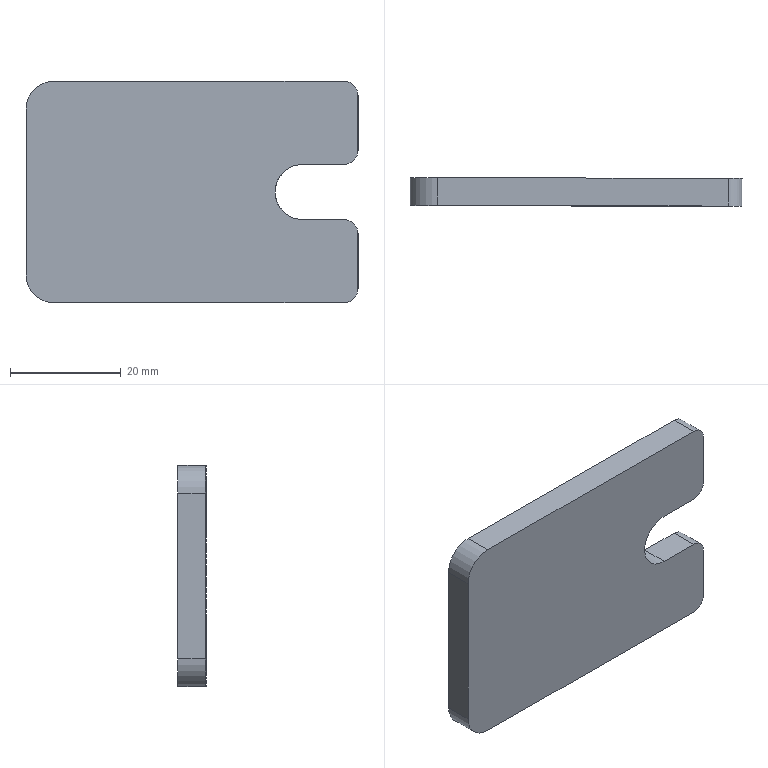Part | STEP file | Input 43 | 1 solid | 16 faces | box 60.015 x 5.178 x 40 mm | volume 11223 mm3 | plane 9 | cylinder 7 | commonest cylinder face diameters 5 x4 10 x3
STEP:
#1=CARTESIAN_POINT('',(0.,0.,0.));
#2=DIRECTION('',(0.,0.,1.));
#3=DIRECTION('',(1.,0.,0.));
#4=AXIS2_PLACEMENT_3D('',#1,#2,#3);
#5=CARTESIAN_POINT('',(-3018.306,387.735,-155.745));
#6=VERTEX_POINT('',#5);
#7=CARTESIAN_POINT('',(-3018.321,382.735,-155.745));
#8=VERTEX_POINT('',#7);
#9=CARTESIAN_POINT('',(-3018.306,387.735,-155.745));
#10=DIRECTION('',(-0.002971,-1.,0.));
#11=VECTOR('',#10,1.);
#12=LINE('',#9,#11);
#13=CARTESIAN_POINT('',(-3018.306,387.735,-160.745));
#14=DIRECTION('',(-0.002971,-1.,0.));
#15=DIRECTION('',(1.,-0.002971,0.));
#16=AXIS2_PLACEMENT_3D('',#13,#14,#15);
#17=CYLINDRICAL_SURFACE('',#16,5.);
#18=CARTESIAN_POINT('',(1.571,0.));
#19=DIRECTION('',(0.,1.));
#20=VECTOR('',#19,1.);
#21=LINE('',#18,#20);
#22=(GEOMETRIC_REPRESENTATION_CONTEXT(2)PARAMETRIC_REPRESENTATION_CONTEXT()REPRESENTATION_CONTEXT('',''));
#23=DEFINITIONAL_REPRESENTATION('',(#21),#22);
#24=PCURVE('',#17,#23);
#25=CARTESIAN_POINT('',(-3018.306,387.735,-155.745));
#26=DIRECTION('',(0.,0.,1.));
#27=DIRECTION('',(1.,-0.002971,0.));
#28=AXIS2_PLACEMENT_3D('',#25,#26,#27);
#29=PLANE('',#28);
#30=CARTESIAN_POINT('',(0.,0.));
#31=DIRECTION('',(0.,-1.));
#32=VECTOR('',#31,1.);
#33=LINE('',#30,#32);
#34=(GEOMETRIC_REPRESENTATION_CONTEXT(2)PARAMETRIC_REPRESENTATION_CONTEXT()REPRESENTATION_CONTEXT('',''));
#35=DEFINITIONAL_REPRESENTATION('',(#33),#34);
#36=PCURVE('',#29,#35);
#37=SURFACE_CURVE('',#12,(#24,#36),.PCURVE_S1.);
#38=EDGE_CURVE('',#6,#8,#37,.T.);
#39=ORIENTED_EDGE('',*,*,#38,.F.);
#40=CARTESIAN_POINT('',(-3018.306,387.735,-165.745));
#41=VERTEX_POINT('',#40);
#42=CARTESIAN_POINT('',(-3018.306,387.735,-160.745));
#43=DIRECTION('',(-0.002971,-1.,0.));
#44=DIRECTION('',(-1.,0.002971,0.));
#45=AXIS2_PLACEMENT_3D('',#42,#43,#44);
#46=CIRCLE('',#45,5.);
#47=CARTESIAN_POINT('',(-3.142,0.));
#48=DIRECTION('',(1.,0.));
#49=VECTOR('',#48,1.);
#50=LINE('',#47,#49);
#51=(GEOMETRIC_REPRESENTATION_CONTEXT(2)PARAMETRIC_REPRESENTATION_CONTEXT()REPRESENTATION_CONTEXT('',''));
#52=DEFINITIONAL_REPRESENTATION('',(#50),#51);
#53=PCURVE('',#17,#52);
#54=CARTESIAN_POINT('',(-3018.306,387.735,-160.745));
#55=DIRECTION('',(0.002971,1.,0.));
#56=DIRECTION('',(-1.,0.002971,0.));
#57=AXIS2_PLACEMENT_3D('',#54,#55,#56);
#58=PLANE('',#57);
#59=CARTESIAN_POINT('',(5.,0.));
#60=CARTESIAN_POINT('',(5.,-8.66));
#61=CARTESIAN_POINT('',(-2.5,-4.33));
#62=CARTESIAN_POINT('',(-10.,0.));
#63=CARTESIAN_POINT('',(-2.5,4.33));
#64=CARTESIAN_POINT('',(5.,8.66));
#65=CARTESIAN_POINT('',(5.,0.));
#66=(BOUNDED_CURVE()B_SPLINE_CURVE(2,(#59,#60,#61,#62,#63,#64,#65),.UNSPECIFIED.,.T.,.F.)B_SPLINE_CURVE_WITH_KNOTS((1,2,2,2,2,1),(-2.094,0.,2.094,4.189,6.283,8.378),.UNSPECIFIED.)CURVE()GEOMETRIC_REPRESENTATION_ITEM()RATIONAL_B_SPLINE_CURVE((1.,0.5,1.,0.5,1.,0.5,1.))REPRESENTATION_ITEM(''));
#67=(GEOMETRIC_REPRESENTATION_CONTEXT(2)PARAMETRIC_REPRESENTATION_CONTEXT()REPRESENTATION_CONTEXT('',''));
#68=DEFINITIONAL_REPRESENTATION('',(#66),#67);
#69=PCURVE('',#58,#68);
#70=SURFACE_CURVE('',#46,(#53,#69),.PCURVE_S1.);
#71=EDGE_CURVE('',#6,#41,#70,.T.);
#72=ORIENTED_EDGE('',*,*,#71,.T.);
#73=CARTESIAN_POINT('',(-3018.321,382.735,-165.745));
#74=VERTEX_POINT('',#73);
#75=CARTESIAN_POINT('',(-3018.306,387.735,-165.745));
#76=DIRECTION('',(-0.002971,-1.,0.));
#77=VECTOR('',#76,1.);
#78=LINE('',#75,#77);
#79=CARTESIAN_POINT('',(4.712,0.));
#80=DIRECTION('',(0.,1.));
#81=VECTOR('',#80,1.);
#82=LINE('',#79,#81);
#83=(GEOMETRIC_REPRESENTATION_CONTEXT(2)PARAMETRIC_REPRESENTATION_CONTEXT()REPRESENTATION_CONTEXT('',''));
#84=DEFINITIONAL_REPRESENTATION('',(#82),#83);
#85=PCURVE('',#17,#84);
#86=CARTESIAN_POINT('',(-3018.306,387.735,-165.745));
#87=DIRECTION('',(0.,0.,-1.));
#88=DIRECTION('',(-1.,0.002971,0.));
#89=AXIS2_PLACEMENT_3D('',#86,#87,#88);
#90=PLANE('',#89);
#91=CARTESIAN_POINT('',(0.,0.));
#92=DIRECTION('',(0.,-1.));
#93=VECTOR('',#92,1.);
#94=LINE('',#91,#93);
#95=(GEOMETRIC_REPRESENTATION_CONTEXT(2)PARAMETRIC_REPRESENTATION_CONTEXT()REPRESENTATION_CONTEXT('',''));
#96=DEFINITIONAL_REPRESENTATION('',(#94),#95);
#97=PCURVE('',#90,#96);
#98=SURFACE_CURVE('',#78,(#85,#97),.PCURVE_S1.);
#99=EDGE_CURVE('',#41,#74,#98,.T.);
#100=ORIENTED_EDGE('',*,*,#99,.T.);
#101=CARTESIAN_POINT('',(-3018.321,382.735,-160.745));
#102=DIRECTION('',(-0.002971,-1.,0.));
#103=DIRECTION('',(-1.,0.002971,0.));
#104=AXIS2_PLACEMENT_3D('',#101,#102,#103);
#105=CIRCLE('',#104,5.);
#106=CARTESIAN_POINT('',(-3.142,5.));
#107=DIRECTION('',(1.,0.));
#108=VECTOR('',#107,1.);
#109=LINE('',#106,#108);
#110=(GEOMETRIC_REPRESENTATION_CONTEXT(2)PARAMETRIC_REPRESENTATION_CONTEXT()REPRESENTATION_CONTEXT('',''));
#111=DEFINITIONAL_REPRESENTATION('',(#109),#110);
#112=PCURVE('',#17,#111);
#113=CARTESIAN_POINT('',(-3018.321,382.735,-160.745));
#114=DIRECTION('',(0.002971,1.,0.));
#115=DIRECTION('',(-1.,0.002971,0.));
#116=AXIS2_PLACEMENT_3D('',#113,#114,#115);
#117=PLANE('',#116);
#118=CARTESIAN_POINT('',(5.,0.));
#119=CARTESIAN_POINT('',(5.,-8.66));
#120=CARTESIAN_POINT('',(-2.5,-4.33));
#121=CARTESIAN_POINT('',(-10.,0.));
#122=CARTESIAN_POINT('',(-2.5,4.33));
#123=CARTESIAN_POINT('',(5.,8.66));
#124=CARTESIAN_POINT('',(5.,0.));
#125=(BOUNDED_CURVE()B_SPLINE_CURVE(2,(#118,#119,#120,#121,#122,#123,#124),.UNSPECIFIED.,.T.,.F.)B_SPLINE_CURVE_WITH_KNOTS((1,2,2,2,2,1),(-2.094,0.,2.094,4.189,6.283,8.378),.UNSPECIFIED.)CURVE()GEOMETRIC_REPRESENTATION_ITEM()RATIONAL_B_SPLINE_CURVE((1.,0.5,1.,0.5,1.,0.5,1.))REPRESENTATION_ITEM(''));
#126=(GEOMETRIC_REPRESENTATION_CONTEXT(2)PARAMETRIC_REPRESENTATION_CONTEXT()REPRESENTATION_CONTEXT('',''));
#127=DEFINITIONAL_REPRESENTATION('',(#125),#126);
#128=PCURVE('',#117,#127);
#129=SURFACE_CURVE('',#105,(#112,#128),.PCURVE_S1.);
#130=EDGE_CURVE('',#8,#74,#129,.T.);
#131=ORIENTED_EDGE('',*,*,#130,.F.);
#132=EDGE_LOOP('',(#39,#72,#100,#131));
#133=FACE_BOUND('',#132,.F.);
#134=ADVANCED_FACE('',(#133),#17,.F.);
#135=CARTESIAN_POINT('',(-3010.821,382.713,-165.745));
#136=VERTEX_POINT('',#135);
#137=CARTESIAN_POINT('',(-3018.321,382.735,-165.745));
#138=DIRECTION('',(1.,-0.002971,0.));
#139=VECTOR('',#138,1.);
#140=LINE('',#137,#139);
#141=CARTESIAN_POINT('',(0.,-5.));
#142=DIRECTION('',(-1.,0.));
#143=VECTOR('',#142,1.);
#144=LINE('',#141,#143);
#145=(GEOMETRIC_REPRESENTATION_CONTEXT(2)PARAMETRIC_REPRESENTATION_CONTEXT()REPRESENTATION_CONTEXT('',''));
#146=DEFINITIONAL_REPRESENTATION('',(#144),#145);
#147=PCURVE('',#90,#146);
#148=CARTESIAN_POINT('',(0.,-5.));
#149=DIRECTION('',(-1.,0.));
#150=VECTOR('',#149,1.);
#151=LINE('',#148,#150);
#152=(GEOMETRIC_REPRESENTATION_CONTEXT(2)PARAMETRIC_REPRESENTATION_CONTEXT()REPRESENTATION_CONTEXT('',''));
#153=DEFINITIONAL_REPRESENTATION('',(#151),#152);
#154=PCURVE('',#117,#153);
#155=SURFACE_CURVE('',#140,(#147,#154),.PCURVE_S1.);
#156=EDGE_CURVE('',#74,#136,#155,.T.);
#157=ORIENTED_EDGE('',*,*,#156,.T.);
#158=CARTESIAN_POINT('',(-3010.806,387.713,-165.745));
#159=VERTEX_POINT('',#158);
#160=CARTESIAN_POINT('',(-3010.806,387.713,-165.745));
#161=DIRECTION('',(-0.002971,-1.,0.));
#162=VECTOR('',#161,1.);
#163=LINE('',#160,#162);
#164=CARTESIAN_POINT('',(-7.5,0.));
#165=DIRECTION('',(0.,-1.));
#166=VECTOR('',#165,1.);
#167=LINE('',#164,#166);
#168=(GEOMETRIC_REPRESENTATION_CONTEXT(2)PARAMETRIC_REPRESENTATION_CONTEXT()REPRESENTATION_CONTEXT('',''));
#169=DEFINITIONAL_REPRESENTATION('',(#167),#168);
#170=PCURVE('',#90,#169);
#171=CARTESIAN_POINT('',(-3010.806,387.713,-168.245));
#172=DIRECTION('',(-0.002971,-1.,0.));
#173=DIRECTION('',(1.,-0.002971,0.));
#174=AXIS2_PLACEMENT_3D('',#171,#172,#173);
#175=CYLINDRICAL_SURFACE('',#174,2.5);
#176=CARTESIAN_POINT('',(1.571,0.));
#177=DIRECTION('',(0.,1.));
#178=VECTOR('',#177,1.);
#179=LINE('',#176,#178);
#180=(GEOMETRIC_REPRESENTATION_CONTEXT(2)PARAMETRIC_REPRESENTATION_CONTEXT()REPRESENTATION_CONTEXT('',''));
#181=DEFINITIONAL_REPRESENTATION('',(#179),#180);
#182=PCURVE('',#175,#181);
#183=SURFACE_CURVE('',#163,(#170,#182),.PCURVE_S1.);
#184=EDGE_CURVE('',#159,#136,#183,.T.);
#185=ORIENTED_EDGE('',*,*,#184,.F.);
#186=CARTESIAN_POINT('',(-3018.306,387.735,-165.745));
#187=DIRECTION('',(1.,-0.002971,0.));
#188=VECTOR('',#187,1.);
#189=LINE('',#186,#188);
#190=CARTESIAN_POINT('',(0.,0.));
#191=DIRECTION('',(-1.,0.));
#192=VECTOR('',#191,1.);
#193=LINE('',#190,#192);
#194=(GEOMETRIC_REPRESENTATION_CONTEXT(2)PARAMETRIC_REPRESENTATION_CONTEXT()REPRESENTATION_CONTEXT('',''));
#195=DEFINITIONAL_REPRESENTATION('',(#193),#194);
#196=PCURVE('',#90,#195);
#197=CARTESIAN_POINT('',(0.,-5.));
#198=DIRECTION('',(-1.,0.));
#199=VECTOR('',#198,1.);
#200=LINE('',#197,#199);
#201=(GEOMETRIC_REPRESENTATION_CONTEXT(2)PARAMETRIC_REPRESENTATION_CONTEXT()REPRESENTATION_CONTEXT('',''));
#202=DEFINITIONAL_REPRESENTATION('',(#200),#201);
#203=PCURVE('',#58,#202);
#204=SURFACE_CURVE('',#189,(#196,#203),.PCURVE_S1.);
#205=EDGE_CURVE('',#41,#159,#204,.T.);
#206=ORIENTED_EDGE('',*,*,#205,.F.);
#207=ORIENTED_EDGE('',*,*,#99,.T.);
#208=EDGE_LOOP('',(#157,#185,#206,#207));
#209=FACE_BOUND('',#208,.T.);
#210=ADVANCED_FACE('',(#209),#90,.F.);
#211=CARTESIAN_POINT('',(-3008.321,382.706,-168.245));
#212=VERTEX_POINT('',#211);
#213=CARTESIAN_POINT('',(-3010.821,382.713,-168.245));
#214=DIRECTION('',(0.002971,1.,0.));
#215=DIRECTION('',(-1.,0.002971,0.));
#216=AXIS2_PLACEMENT_3D('',#213,#214,#215);
#217=CIRCLE('',#216,2.5);
#218=CARTESIAN_POINT('',(3.142,5.));
#219=DIRECTION('',(-1.,0.));
#220=VECTOR('',#219,1.);
#221=LINE('',#218,#220);
#222=(GEOMETRIC_REPRESENTATION_CONTEXT(2)PARAMETRIC_REPRESENTATION_CONTEXT()REPRESENTATION_CONTEXT('',''));
#223=DEFINITIONAL_REPRESENTATION('',(#221),#222);
#224=PCURVE('',#175,#223);
#225=CARTESIAN_POINT('',(-7.5,-7.5));
#226=DIRECTION('',(1.,0.));
#227=AXIS2_PLACEMENT_2D('',#225,#226);
#228=CIRCLE('',#227,2.5);
#229=(GEOMETRIC_REPRESENTATION_CONTEXT(2)PARAMETRIC_REPRESENTATION_CONTEXT()REPRESENTATION_CONTEXT('',''));
#230=DEFINITIONAL_REPRESENTATION('',(#228),#229);
#231=PCURVE('',#117,#230);
#232=SURFACE_CURVE('',#217,(#224,#231),.PCURVE_S1.);
#233=EDGE_CURVE('',#136,#212,#232,.T.);
#234=ORIENTED_EDGE('',*,*,#233,.T.);
#235=CARTESIAN_POINT('',(-3008.306,387.705,-168.245));
#236=VERTEX_POINT('',#235);
#237=CARTESIAN_POINT('',(-3008.306,387.705,-168.245));
#238=DIRECTION('',(-0.002971,-1.,0.));
#239=VECTOR('',#238,1.);
#240=LINE('',#237,#239);
#241=CARTESIAN_POINT('',(0.,0.));
#242=DIRECTION('',(0.,1.));
#243=VECTOR('',#242,1.);
#244=LINE('',#241,#243);
#245=(GEOMETRIC_REPRESENTATION_CONTEXT(2)PARAMETRIC_REPRESENTATION_CONTEXT()REPRESENTATION_CONTEXT('',''));
#246=DEFINITIONAL_REPRESENTATION('',(#244),#245);
#247=PCURVE('',#175,#246);
#248=CARTESIAN_POINT('',(-3008.306,387.705,-168.245));
#249=DIRECTION('',(-1.,0.002971,0.));
#250=DIRECTION('',(0.,0.,1.));
#251=AXIS2_PLACEMENT_3D('',#248,#249,#250);
#252=PLANE('',#251);
#253=CARTESIAN_POINT('',(0.,0.));
#254=DIRECTION('',(0.,-1.));
#255=VECTOR('',#254,1.);
#256=LINE('',#253,#255);
#257=(GEOMETRIC_REPRESENTATION_CONTEXT(2)PARAMETRIC_REPRESENTATION_CONTEXT()REPRESENTATION_CONTEXT('',''));
#258=DEFINITIONAL_REPRESENTATION('',(#256),#257);
#259=PCURVE('',#252,#258);
#260=SURFACE_CURVE('',#240,(#247,#259),.PCURVE_S1.);
#261=EDGE_CURVE('',#236,#212,#260,.T.);
#262=ORIENTED_EDGE('',*,*,#261,.F.);
#263=CARTESIAN_POINT('',(-3010.806,387.713,-168.245));
#264=DIRECTION('',(0.002971,1.,0.));
#265=DIRECTION('',(-1.,0.002971,0.));
#266=AXIS2_PLACEMENT_3D('',#263,#264,#265);
#267=CIRCLE('',#266,2.5);
#268=CARTESIAN_POINT('',(3.142,0.));
#269=DIRECTION('',(-1.,0.));
#270=VECTOR('',#269,1.);
#271=LINE('',#268,#270);
#272=(GEOMETRIC_REPRESENTATION_CONTEXT(2)PARAMETRIC_REPRESENTATION_CONTEXT()REPRESENTATION_CONTEXT('',''));
#273=DEFINITIONAL_REPRESENTATION('',(#271),#272);
#274=PCURVE('',#175,#273);
#275=CARTESIAN_POINT('',(-7.5,-7.5));
#276=DIRECTION('',(1.,0.));
#277=AXIS2_PLACEMENT_2D('',#275,#276);
#278=CIRCLE('',#277,2.5);
#279=(GEOMETRIC_REPRESENTATION_CONTEXT(2)PARAMETRIC_REPRESENTATION_CONTEXT()REPRESENTATION_CONTEXT('',''));
#280=DEFINITIONAL_REPRESENTATION('',(#278),#279);
#281=PCURVE('',#58,#280);
#282=SURFACE_CURVE('',#267,(#274,#281),.PCURVE_S1.);
#283=EDGE_CURVE('',#159,#236,#282,.T.);
#284=ORIENTED_EDGE('',*,*,#283,.F.);
#285=ORIENTED_EDGE('',*,*,#184,.T.);
#286=EDGE_LOOP('',(#234,#262,#284,#285));
#287=FACE_BOUND('',#286,.T.);
#288=ADVANCED_FACE('',(#287),#175,.T.);
#289=CARTESIAN_POINT('',(-3008.321,382.706,-178.245));
#290=VERTEX_POINT('',#289);
#291=CARTESIAN_POINT('',(-3008.321,382.706,-168.245));
#292=DIRECTION('',(0.,0.,-1.));
#293=VECTOR('',#292,1.);
#294=LINE('',#291,#293);
#295=CARTESIAN_POINT('',(0.,-5.));
#296=DIRECTION('',(-1.,0.));
#297=VECTOR('',#296,1.);
#298=LINE('',#295,#297);
#299=(GEOMETRIC_REPRESENTATION_CONTEXT(2)PARAMETRIC_REPRESENTATION_CONTEXT()REPRESENTATION_CONTEXT('',''));
#300=DEFINITIONAL_REPRESENTATION('',(#298),#299);
#301=PCURVE('',#252,#300);
#302=CARTESIAN_POINT('',(-10.,-7.5));
#303=DIRECTION('',(0.,-1.));
#304=VECTOR('',#303,1.);
#305=LINE('',#302,#304);
#306=(GEOMETRIC_REPRESENTATION_CONTEXT(2)PARAMETRIC_REPRESENTATION_CONTEXT()REPRESENTATION_CONTEXT('',''));
#307=DEFINITIONAL_REPRESENTATION('',(#305),#306);
#308=PCURVE('',#117,#307);
#309=SURFACE_CURVE('',#294,(#301,#308),.PCURVE_S1.);
#310=EDGE_CURVE('',#212,#290,#309,.T.);
#311=ORIENTED_EDGE('',*,*,#310,.T.);
#312=CARTESIAN_POINT('',(-3008.306,387.705,-178.245));
#313=VERTEX_POINT('',#312);
#314=CARTESIAN_POINT('',(-3008.306,387.705,-178.245));
#315=DIRECTION('',(-0.002971,-1.,0.));
#316=VECTOR('',#315,1.);
#317=LINE('',#314,#316);
#318=CARTESIAN_POINT('',(-10.,0.));
#319=DIRECTION('',(0.,-1.));
#320=VECTOR('',#319,1.);
#321=LINE('',#318,#320);
#322=(GEOMETRIC_REPRESENTATION_CONTEXT(2)PARAMETRIC_REPRESENTATION_CONTEXT()REPRESENTATION_CONTEXT('',''));
#323=DEFINITIONAL_REPRESENTATION('',(#321),#322);
#324=PCURVE('',#252,#323);
#325=CARTESIAN_POINT('',(-3010.806,387.713,-178.245));
#326=DIRECTION('',(-0.002971,-1.,0.));
#327=DIRECTION('',(1.,-0.002971,0.));
#328=AXIS2_PLACEMENT_3D('',#325,#326,#327);
#329=CYLINDRICAL_SURFACE('',#328,2.5);
#330=CARTESIAN_POINT('',(6.283,0.));
#331=DIRECTION('',(0.,1.));
#332=VECTOR('',#331,1.);
#333=LINE('',#330,#332);
#334=(GEOMETRIC_REPRESENTATION_CONTEXT(2)PARAMETRIC_REPRESENTATION_CONTEXT()REPRESENTATION_CONTEXT('',''));
#335=DEFINITIONAL_REPRESENTATION('',(#333),#334);
#336=PCURVE('',#329,#335);
#337=SURFACE_CURVE('',#317,(#324,#336),.PCURVE_S1.);
#338=EDGE_CURVE('',#313,#290,#337,.T.);
#339=ORIENTED_EDGE('',*,*,#338,.F.);
#340=CARTESIAN_POINT('',(-3008.306,387.705,-168.245));
#341=DIRECTION('',(0.,0.,-1.));
#342=VECTOR('',#341,1.);
#343=LINE('',#340,#342);
#344=CARTESIAN_POINT('',(0.,0.));
#345=DIRECTION('',(-1.,0.));
#346=VECTOR('',#345,1.);
#347=LINE('',#344,#346);
#348=(GEOMETRIC_REPRESENTATION_CONTEXT(2)PARAMETRIC_REPRESENTATION_CONTEXT()REPRESENTATION_CONTEXT('',''));
#349=DEFINITIONAL_REPRESENTATION('',(#347),#348);
#350=PCURVE('',#252,#349);
#351=CARTESIAN_POINT('',(-10.,-7.5));
#352=DIRECTION('',(0.,-1.));
#353=VECTOR('',#352,1.);
#354=LINE('',#351,#353);
#355=(GEOMETRIC_REPRESENTATION_CONTEXT(2)PARAMETRIC_REPRESENTATION_CONTEXT()REPRESENTATION_CONTEXT('',''));
#356=DEFINITIONAL_REPRESENTATION('',(#354),#355);
#357=PCURVE('',#58,#356);
#358=SURFACE_CURVE('',#343,(#350,#357),.PCURVE_S1.);
#359=EDGE_CURVE('',#236,#313,#358,.T.);
#360=ORIENTED_EDGE('',*,*,#359,.F.);
#361=ORIENTED_EDGE('',*,*,#261,.T.);
#362=EDGE_LOOP('',(#311,#339,#360,#361));
#363=FACE_BOUND('',#362,.T.);
#364=ADVANCED_FACE('',(#363),#252,.F.);
#365=CARTESIAN_POINT('',(-3010.821,382.713,-180.745));
#366=VERTEX_POINT('',#365);
#367=CARTESIAN_POINT('',(-3010.821,382.713,-178.245));
#368=DIRECTION('',(0.002971,1.,0.));
#369=DIRECTION('',(-1.,0.002971,0.));
#370=AXIS2_PLACEMENT_3D('',#367,#368,#369);
#371=CIRCLE('',#370,2.5);
#372=CARTESIAN_POINT('',(9.425,5.));
#373=DIRECTION('',(-1.,0.));
#374=VECTOR('',#373,1.);
#375=LINE('',#372,#374);
#376=(GEOMETRIC_REPRESENTATION_CONTEXT(2)PARAMETRIC_REPRESENTATION_CONTEXT()REPRESENTATION_CONTEXT('',''));
#377=DEFINITIONAL_REPRESENTATION('',(#375),#376);
#378=PCURVE('',#329,#377);
#379=CARTESIAN_POINT('',(-7.5,-17.5));
#380=DIRECTION('',(1.,0.));
#381=AXIS2_PLACEMENT_2D('',#379,#380);
#382=CIRCLE('',#381,2.5);
#383=(GEOMETRIC_REPRESENTATION_CONTEXT(2)PARAMETRIC_REPRESENTATION_CONTEXT()REPRESENTATION_CONTEXT('',''));
#384=DEFINITIONAL_REPRESENTATION('',(#382),#383);
#385=PCURVE('',#117,#384);
#386=SURFACE_CURVE('',#371,(#378,#385),.PCURVE_S1.);
#387=EDGE_CURVE('',#290,#366,#386,.T.);
#388=ORIENTED_EDGE('',*,*,#387,.T.);
#389=CARTESIAN_POINT('',(-3010.806,387.713,-180.745));
#390=VERTEX_POINT('',#389);
#391=CARTESIAN_POINT('',(-3010.806,387.713,-180.745));
#392=DIRECTION('',(-0.002971,-1.,0.));
#393=VECTOR('',#392,1.);
#394=LINE('',#391,#393);
#395=CARTESIAN_POINT('',(4.712,0.));
#396=DIRECTION('',(0.,1.));
#397=VECTOR('',#396,1.);
#398=LINE('',#395,#397);
#399=(GEOMETRIC_REPRESENTATION_CONTEXT(2)PARAMETRIC_REPRESENTATION_CONTEXT()REPRESENTATION_CONTEXT('',''));
#400=DEFINITIONAL_REPRESENTATION('',(#398),#399);
#401=PCURVE('',#329,#400);
#402=CARTESIAN_POINT('',(-3010.806,387.713,-180.745));
#403=DIRECTION('',(0.,0.,1.));
#404=DIRECTION('',(1.,-0.002971,0.));
#405=AXIS2_PLACEMENT_3D('',#402,#403,#404);
#406=PLANE('',#405);
#407=CARTESIAN_POINT('',(0.,0.));
#408=DIRECTION('',(0.,-1.));
#409=VECTOR('',#408,1.);
#410=LINE('',#407,#409);
#411=(GEOMETRIC_REPRESENTATION_CONTEXT(2)PARAMETRIC_REPRESENTATION_CONTEXT()REPRESENTATION_CONTEXT('',''));
#412=DEFINITIONAL_REPRESENTATION('',(#410),#411);
#413=PCURVE('',#406,#412);
#414=SURFACE_CURVE('',#394,(#401,#413),.PCURVE_S1.);
#415=EDGE_CURVE('',#390,#366,#414,.T.);
#416=ORIENTED_EDGE('',*,*,#415,.F.);
#417=CARTESIAN_POINT('',(-3010.806,387.713,-178.245));
#418=DIRECTION('',(0.002971,1.,0.));
#419=DIRECTION('',(-1.,0.002971,0.));
#420=AXIS2_PLACEMENT_3D('',#417,#418,#419);
#421=CIRCLE('',#420,2.5);
#422=CARTESIAN_POINT('',(9.425,0.));
#423=DIRECTION('',(-1.,0.));
#424=VECTOR('',#423,1.);
#425=LINE('',#422,#424);
#426=(GEOMETRIC_REPRESENTATION_CONTEXT(2)PARAMETRIC_REPRESENTATION_CONTEXT()REPRESENTATION_CONTEXT('',''));
#427=DEFINITIONAL_REPRESENTATION('',(#425),#426);
#428=PCURVE('',#329,#427);
#429=CARTESIAN_POINT('',(-7.5,-17.5));
#430=DIRECTION('',(1.,0.));
#431=AXIS2_PLACEMENT_2D('',#429,#430);
#432=CIRCLE('',#431,2.5);
#433=(GEOMETRIC_REPRESENTATION_CONTEXT(2)PARAMETRIC_REPRESENTATION_CONTEXT()REPRESENTATION_CONTEXT('',''));
#434=DEFINITIONAL_REPRESENTATION('',(#432),#433);
#435=PCURVE('',#58,#434);
#436=SURFACE_CURVE('',#421,(#428,#435),.PCURVE_S1.);
#437=EDGE_CURVE('',#313,#390,#436,.T.);
#438=ORIENTED_EDGE('',*,*,#437,.F.);
#439=ORIENTED_EDGE('',*,*,#338,.T.);
#440=EDGE_LOOP('',(#388,#416,#438,#439));
#441=FACE_BOUND('',#440,.T.);
#442=ADVANCED_FACE('',(#441),#329,.T.);
#443=CARTESIAN_POINT('',(-3063.321,382.869,-180.745));
#444=VERTEX_POINT('',#443);
#445=CARTESIAN_POINT('',(-3010.821,382.713,-180.745));
#446=DIRECTION('',(-1.,0.002971,0.));
#447=VECTOR('',#446,1.);
#448=LINE('',#445,#447);
#449=CARTESIAN_POINT('',(0.,-5.));
#450=DIRECTION('',(-1.,0.));
#451=VECTOR('',#450,1.);
#452=LINE('',#449,#451);
#453=(GEOMETRIC_REPRESENTATION_CONTEXT(2)PARAMETRIC_REPRESENTATION_CONTEXT()REPRESENTATION_CONTEXT('',''));
#454=DEFINITIONAL_REPRESENTATION('',(#452),#453);
#455=PCURVE('',#406,#454);
#456=CARTESIAN_POINT('',(-7.5,-20.));
#457=DIRECTION('',(1.,0.));
#458=VECTOR('',#457,1.);
#459=LINE('',#456,#458);
#460=(GEOMETRIC_REPRESENTATION_CONTEXT(2)PARAMETRIC_REPRESENTATION_CONTEXT()REPRESENTATION_CONTEXT('',''));
#461=DEFINITIONAL_REPRESENTATION('',(#459),#460);
#462=PCURVE('',#117,#461);
#463=SURFACE_CURVE('',#448,(#455,#462),.PCURVE_S1.);
#464=EDGE_CURVE('',#366,#444,#463,.T.);
#465=ORIENTED_EDGE('',*,*,#464,.T.);
#466=CARTESIAN_POINT('',(-3063.306,387.869,-180.745));
#467=VERTEX_POINT('',#466);
#468=CARTESIAN_POINT('',(-3063.306,387.869,-180.745));
#469=DIRECTION('',(-0.002971,-1.,0.));
#470=VECTOR('',#469,1.);
#471=LINE('',#468,#470);
#472=CARTESIAN_POINT('',(-52.5,0.));
#473=DIRECTION('',(0.,-1.));
#474=VECTOR('',#473,1.);
#475=LINE('',#472,#474);
#476=(GEOMETRIC_REPRESENTATION_CONTEXT(2)PARAMETRIC_REPRESENTATION_CONTEXT()REPRESENTATION_CONTEXT('',''));
#477=DEFINITIONAL_REPRESENTATION('',(#475),#476);
#478=PCURVE('',#406,#477);
#479=CARTESIAN_POINT('',(-3063.306,387.869,-175.745));
#480=DIRECTION('',(-0.002971,-1.,0.));
#481=DIRECTION('',(1.,-0.002971,0.));
#482=AXIS2_PLACEMENT_3D('',#479,#480,#481);
#483=CYLINDRICAL_SURFACE('',#482,5.);
#484=CARTESIAN_POINT('',(4.712,0.));
#485=DIRECTION('',(0.,1.));
#486=VECTOR('',#485,1.);
#487=LINE('',#484,#486);
#488=(GEOMETRIC_REPRESENTATION_CONTEXT(2)PARAMETRIC_REPRESENTATION_CONTEXT()REPRESENTATION_CONTEXT('',''));
#489=DEFINITIONAL_REPRESENTATION('',(#487),#488);
#490=PCURVE('',#483,#489);
#491=SURFACE_CURVE('',#471,(#478,#490),.PCURVE_S1.);
#492=EDGE_CURVE('',#467,#444,#491,.T.);
#493=ORIENTED_EDGE('',*,*,#492,.F.);
#494=CARTESIAN_POINT('',(-3010.806,387.713,-180.745));
#495=DIRECTION('',(-1.,0.002971,0.));
#496=VECTOR('',#495,1.);
#497=LINE('',#494,#496);
#498=CARTESIAN_POINT('',(0.,0.));
#499=DIRECTION('',(-1.,0.));
#500=VECTOR('',#499,1.);
#501=LINE('',#498,#500);
#502=(GEOMETRIC_REPRESENTATION_CONTEXT(2)PARAMETRIC_REPRESENTATION_CONTEXT()REPRESENTATION_CONTEXT('',''));
#503=DEFINITIONAL_REPRESENTATION('',(#501),#502);
#504=PCURVE('',#406,#503);
#505=CARTESIAN_POINT('',(-7.5,-20.));
#506=DIRECTION('',(1.,0.));
#507=VECTOR('',#506,1.);
#508=LINE('',#505,#507);
#509=(GEOMETRIC_REPRESENTATION_CONTEXT(2)PARAMETRIC_REPRESENTATION_CONTEXT()REPRESENTATION_CONTEXT('',''));
#510=DEFINITIONAL_REPRESENTATION('',(#508),#509);
#511=PCURVE('',#58,#510);
#512=SURFACE_CURVE('',#497,(#504,#511),.PCURVE_S1.);
#513=EDGE_CURVE('',#390,#467,#512,.T.);
#514=ORIENTED_EDGE('',*,*,#513,.F.);
#515=ORIENTED_EDGE('',*,*,#415,.T.);
#516=EDGE_LOOP('',(#465,#493,#514,#515));
#517=FACE_BOUND('',#516,.T.);
#518=ADVANCED_FACE('',(#517),#406,.F.);
#519=CARTESIAN_POINT('',(-3068.321,382.884,-175.745));
#520=VERTEX_POINT('',#519);
#521=CARTESIAN_POINT('',(-3063.321,382.869,-175.745));
#522=DIRECTION('',(0.002971,1.,0.));
#523=DIRECTION('',(1.,-0.002971,0.));
#524=AXIS2_PLACEMENT_3D('',#521,#522,#523);
#525=CIRCLE('',#524,5.);
#526=CARTESIAN_POINT('',(6.283,5.));
#527=DIRECTION('',(-1.,0.));
#528=VECTOR('',#527,1.);
#529=LINE('',#526,#528);
#530=(GEOMETRIC_REPRESENTATION_CONTEXT(2)PARAMETRIC_REPRESENTATION_CONTEXT()REPRESENTATION_CONTEXT('',''));
#531=DEFINITIONAL_REPRESENTATION('',(#529),#530);
#532=PCURVE('',#483,#531);
#533=CARTESIAN_POINT('',(45.,-15.));
#534=DIRECTION('',(-1.,0.));
#535=AXIS2_PLACEMENT_2D('',#533,#534);
#536=CIRCLE('',#535,5.);
#537=(GEOMETRIC_REPRESENTATION_CONTEXT(2)PARAMETRIC_REPRESENTATION_CONTEXT()REPRESENTATION_CONTEXT('',''));
#538=DEFINITIONAL_REPRESENTATION('',(#536),#537);
#539=PCURVE('',#117,#538);
#540=SURFACE_CURVE('',#525,(#532,#539),.PCURVE_S1.);
#541=EDGE_CURVE('',#444,#520,#540,.T.);
#542=ORIENTED_EDGE('',*,*,#541,.T.);
#543=CARTESIAN_POINT('',(-3068.306,387.884,-175.745));
#544=VERTEX_POINT('',#543);
#545=CARTESIAN_POINT('',(-3068.306,387.884,-175.745));
#546=DIRECTION('',(-0.002971,-1.,0.));
#547=VECTOR('',#546,1.);
#548=LINE('',#545,#547);
#549=CARTESIAN_POINT('',(3.142,0.));
#550=DIRECTION('',(0.,1.));
#551=VECTOR('',#550,1.);
#552=LINE('',#549,#551);
#553=(GEOMETRIC_REPRESENTATION_CONTEXT(2)PARAMETRIC_REPRESENTATION_CONTEXT()REPRESENTATION_CONTEXT('',''));
#554=DEFINITIONAL_REPRESENTATION('',(#552),#553);
#555=PCURVE('',#483,#554);
#556=CARTESIAN_POINT('',(-3068.306,387.884,-175.745));
#557=DIRECTION('',(1.,-0.002971,0.));
#558=DIRECTION('',(0.,0.,-1.));
#559=AXIS2_PLACEMENT_3D('',#556,#557,#558);
#560=PLANE('',#559);
#561=CARTESIAN_POINT('',(0.,0.));
#562=DIRECTION('',(0.,-1.));
#563=VECTOR('',#562,1.);
#564=LINE('',#561,#563);
#565=(GEOMETRIC_REPRESENTATION_CONTEXT(2)PARAMETRIC_REPRESENTATION_CONTEXT()REPRESENTATION_CONTEXT('',''));
#566=DEFINITIONAL_REPRESENTATION('',(#564),#565);
#567=PCURVE('',#560,#566);
#568=SURFACE_CURVE('',#548,(#555,#567),.PCURVE_S1.);
#569=EDGE_CURVE('',#544,#520,#568,.T.);
#570=ORIENTED_EDGE('',*,*,#569,.F.);
#571=CARTESIAN_POINT('',(-3063.306,387.869,-175.745));
#572=DIRECTION('',(0.002971,1.,0.));
#573=DIRECTION('',(1.,-0.002971,0.));
#574=AXIS2_PLACEMENT_3D('',#571,#572,#573);
#575=CIRCLE('',#574,5.);
#576=CARTESIAN_POINT('',(6.283,0.));
#577=DIRECTION('',(-1.,0.));
#578=VECTOR('',#577,1.);
#579=LINE('',#576,#578);
#580=(GEOMETRIC_REPRESENTATION_CONTEXT(2)PARAMETRIC_REPRESENTATION_CONTEXT()REPRESENTATION_CONTEXT('',''));
#581=DEFINITIONAL_REPRESENTATION('',(#579),#580);
#582=PCURVE('',#483,#581);
#583=CARTESIAN_POINT('',(45.,-15.));
#584=DIRECTION('',(-1.,0.));
#585=AXIS2_PLACEMENT_2D('',#583,#584);
#586=CIRCLE('',#585,5.);
#587=(GEOMETRIC_REPRESENTATION_CONTEXT(2)PARAMETRIC_REPRESENTATION_CONTEXT()REPRESENTATION_CONTEXT('',''));
#588=DEFINITIONAL_REPRESENTATION('',(#586),#587);
#589=PCURVE('',#58,#588);
#590=SURFACE_CURVE('',#575,(#582,#589),.PCURVE_S1.);
#591=EDGE_CURVE('',#467,#544,#590,.T.);
#592=ORIENTED_EDGE('',*,*,#591,.F.);
#593=ORIENTED_EDGE('',*,*,#492,.T.);
#594=EDGE_LOOP('',(#542,#570,#592,#593));
#595=FACE_BOUND('',#594,.T.);
#596=ADVANCED_FACE('',(#595),#483,.T.);
#597=CARTESIAN_POINT('',(-3068.321,382.884,-145.745));
#598=VERTEX_POINT('',#597);
#599=CARTESIAN_POINT('',(-3068.321,382.884,-175.745));
#600=DIRECTION('',(0.,0.,1.));
#601=VECTOR('',#600,1.);
#602=LINE('',#599,#601);
#603=CARTESIAN_POINT('',(0.,-5.));
#604=DIRECTION('',(-1.,0.));
#605=VECTOR('',#604,1.);
#606=LINE('',#603,#605);
#607=(GEOMETRIC_REPRESENTATION_CONTEXT(2)PARAMETRIC_REPRESENTATION_CONTEXT()REPRESENTATION_CONTEXT('',''));
#608=DEFINITIONAL_REPRESENTATION('',(#606),#607);
#609=PCURVE('',#560,#608);
#610=CARTESIAN_POINT('',(50.,-15.));
#611=DIRECTION('',(0.,1.));
#612=VECTOR('',#611,1.);
#613=LINE('',#610,#612);
#614=(GEOMETRIC_REPRESENTATION_CONTEXT(2)PARAMETRIC_REPRESENTATION_CONTEXT()REPRESENTATION_CONTEXT('',''));
#615=DEFINITIONAL_REPRESENTATION('',(#613),#614);
#616=PCURVE('',#117,#615);
#617=SURFACE_CURVE('',#602,(#609,#616),.PCURVE_S1.);
#618=EDGE_CURVE('',#520,#598,#617,.T.);
#619=ORIENTED_EDGE('',*,*,#618,.T.);
#620=CARTESIAN_POINT('',(-3068.306,387.884,-145.745));
#621=VERTEX_POINT('',#620);
#622=CARTESIAN_POINT('',(-3068.306,387.884,-145.745));
#623=DIRECTION('',(-0.002971,-1.,0.));
#624=VECTOR('',#623,1.);
#625=LINE('',#622,#624);
#626=CARTESIAN_POINT('',(-30.,0.));
#627=DIRECTION('',(0.,-1.));
#628=VECTOR('',#627,1.);
#629=LINE('',#626,#628);
#630=(GEOMETRIC_REPRESENTATION_CONTEXT(2)PARAMETRIC_REPRESENTATION_CONTEXT()REPRESENTATION_CONTEXT('',''));
#631=DEFINITIONAL_REPRESENTATION('',(#629),#630);
#632=PCURVE('',#560,#631);
#633=CARTESIAN_POINT('',(-3063.306,387.869,-145.745));
#634=DIRECTION('',(-0.002971,-1.,0.));
#635=DIRECTION('',(1.,-0.002971,0.));
#636=AXIS2_PLACEMENT_3D('',#633,#634,#635);
#637=CYLINDRICAL_SURFACE('',#636,5.);
#638=CARTESIAN_POINT('',(3.142,0.));
#639=DIRECTION('',(0.,1.));
#640=VECTOR('',#639,1.);
#641=LINE('',#638,#640);
#642=(GEOMETRIC_REPRESENTATION_CONTEXT(2)PARAMETRIC_REPRESENTATION_CONTEXT()REPRESENTATION_CONTEXT('',''));
#643=DEFINITIONAL_REPRESENTATION('',(#641),#642);
#644=PCURVE('',#637,#643);
#645=SURFACE_CURVE('',#625,(#632,#644),.PCURVE_S1.);
#646=EDGE_CURVE('',#621,#598,#645,.T.);
#647=ORIENTED_EDGE('',*,*,#646,.F.);
#648=CARTESIAN_POINT('',(-3068.306,387.884,-175.745));
#649=DIRECTION('',(0.,0.,1.));
#650=VECTOR('',#649,1.);
#651=LINE('',#648,#650);
#652=CARTESIAN_POINT('',(0.,0.));
#653=DIRECTION('',(-1.,0.));
#654=VECTOR('',#653,1.);
#655=LINE('',#652,#654);
#656=(GEOMETRIC_REPRESENTATION_CONTEXT(2)PARAMETRIC_REPRESENTATION_CONTEXT()REPRESENTATION_CONTEXT('',''));
#657=DEFINITIONAL_REPRESENTATION('',(#655),#656);
#658=PCURVE('',#560,#657);
#659=CARTESIAN_POINT('',(50.,-15.));
#660=DIRECTION('',(0.,1.));
#661=VECTOR('',#660,1.);
#662=LINE('',#659,#661);
#663=(GEOMETRIC_REPRESENTATION_CONTEXT(2)PARAMETRIC_REPRESENTATION_CONTEXT()REPRESENTATION_CONTEXT('',''));
#664=DEFINITIONAL_REPRESENTATION('',(#662),#663);
#665=PCURVE('',#58,#664);
#666=SURFACE_CURVE('',#651,(#658,#665),.PCURVE_S1.);
#667=EDGE_CURVE('',#544,#621,#666,.T.);
#668=ORIENTED_EDGE('',*,*,#667,.F.);
#669=ORIENTED_EDGE('',*,*,#569,.T.);
#670=EDGE_LOOP('',(#619,#647,#668,#669));
#671=FACE_BOUND('',#670,.T.);
#672=ADVANCED_FACE('',(#671),#560,.F.);
#673=CARTESIAN_POINT('',(-3063.321,382.869,-140.745));
#674=VERTEX_POINT('',#673);
#675=CARTESIAN_POINT('',(-3063.321,382.869,-145.745));
#676=DIRECTION('',(0.002971,1.,0.));
#677=DIRECTION('',(-1.,0.002971,0.));
#678=AXIS2_PLACEMENT_3D('',#675,#676,#677);
#679=CIRCLE('',#678,5.);
#680=CARTESIAN_POINT('',(3.142,5.));
#681=DIRECTION('',(-1.,0.));
#682=VECTOR('',#681,1.);
#683=LINE('',#680,#682);
#684=(GEOMETRIC_REPRESENTATION_CONTEXT(2)PARAMETRIC_REPRESENTATION_CONTEXT()REPRESENTATION_CONTEXT('',''));
#685=DEFINITIONAL_REPRESENTATION('',(#683),#684);
#686=PCURVE('',#637,#685);
#687=CARTESIAN_POINT('',(45.,15.));
#688=DIRECTION('',(1.,0.));
#689=AXIS2_PLACEMENT_2D('',#687,#688);
#690=CIRCLE('',#689,5.);
#691=(GEOMETRIC_REPRESENTATION_CONTEXT(2)PARAMETRIC_REPRESENTATION_CONTEXT()REPRESENTATION_CONTEXT('',''));
#692=DEFINITIONAL_REPRESENTATION('',(#690),#691);
#693=PCURVE('',#117,#692);
#694=SURFACE_CURVE('',#679,(#686,#693),.PCURVE_S1.);
#695=EDGE_CURVE('',#598,#674,#694,.T.);
#696=ORIENTED_EDGE('',*,*,#695,.T.);
#697=CARTESIAN_POINT('',(-3063.306,387.869,-140.745));
#698=VERTEX_POINT('',#697);
#699=CARTESIAN_POINT('',(-3063.306,387.869,-140.745));
#700=DIRECTION('',(-0.002971,-1.,0.));
#701=VECTOR('',#700,1.);
#702=LINE('',#699,#701);
#703=CARTESIAN_POINT('',(1.571,0.));
#704=DIRECTION('',(0.,1.));
#705=VECTOR('',#704,1.);
#706=LINE('',#703,#705);
#707=(GEOMETRIC_REPRESENTATION_CONTEXT(2)PARAMETRIC_REPRESENTATION_CONTEXT()REPRESENTATION_CONTEXT('',''));
#708=DEFINITIONAL_REPRESENTATION('',(#706),#707);
#709=PCURVE('',#637,#708);
#710=CARTESIAN_POINT('',(-3063.306,387.869,-140.745));
#711=DIRECTION('',(0.,0.,-1.));
#712=DIRECTION('',(-1.,0.002971,0.));
#713=AXIS2_PLACEMENT_3D('',#710,#711,#712);
#714=PLANE('',#713);
#715=CARTESIAN_POINT('',(0.,0.));
#716=DIRECTION('',(0.,-1.));
#717=VECTOR('',#716,1.);
#718=LINE('',#715,#717);
#719=(GEOMETRIC_REPRESENTATION_CONTEXT(2)PARAMETRIC_REPRESENTATION_CONTEXT()REPRESENTATION_CONTEXT('',''));
#720=DEFINITIONAL_REPRESENTATION('',(#718),#719);
#721=PCURVE('',#714,#720);
#722=SURFACE_CURVE('',#702,(#709,#721),.PCURVE_S1.);
#723=EDGE_CURVE('',#698,#674,#722,.T.);
#724=ORIENTED_EDGE('',*,*,#723,.F.);
#725=CARTESIAN_POINT('',(-3063.306,387.869,-145.745));
#726=DIRECTION('',(0.002971,1.,0.));
#727=DIRECTION('',(-1.,0.002971,0.));
#728=AXIS2_PLACEMENT_3D('',#725,#726,#727);
#729=CIRCLE('',#728,5.);
#730=CARTESIAN_POINT('',(3.142,0.));
#731=DIRECTION('',(-1.,0.));
#732=VECTOR('',#731,1.);
#733=LINE('',#730,#732);
#734=(GEOMETRIC_REPRESENTATION_CONTEXT(2)PARAMETRIC_REPRESENTATION_CONTEXT()REPRESENTATION_CONTEXT('',''));
#735=DEFINITIONAL_REPRESENTATION('',(#733),#734);
#736=PCURVE('',#637,#735);
#737=CARTESIAN_POINT('',(45.,15.));
#738=DIRECTION('',(1.,0.));
#739=AXIS2_PLACEMENT_2D('',#737,#738);
#740=CIRCLE('',#739,5.);
#741=(GEOMETRIC_REPRESENTATION_CONTEXT(2)PARAMETRIC_REPRESENTATION_CONTEXT()REPRESENTATION_CONTEXT('',''));
#742=DEFINITIONAL_REPRESENTATION('',(#740),#741);
#743=PCURVE('',#58,#742);
#744=SURFACE_CURVE('',#729,(#736,#743),.PCURVE_S1.);
#745=EDGE_CURVE('',#621,#698,#744,.T.);
#746=ORIENTED_EDGE('',*,*,#745,.F.);
#747=ORIENTED_EDGE('',*,*,#646,.T.);
#748=EDGE_LOOP('',(#696,#724,#746,#747));
#749=FACE_BOUND('',#748,.T.);
#750=ADVANCED_FACE('',(#749),#637,.T.);
#751=CARTESIAN_POINT('',(-3010.821,382.713,-140.745));
#752=VERTEX_POINT('',#751);
#753=CARTESIAN_POINT('',(-3063.321,382.869,-140.745));
#754=DIRECTION('',(1.,-0.002971,0.));
#755=VECTOR('',#754,1.);
#756=LINE('',#753,#755);
#757=CARTESIAN_POINT('',(0.,-5.));
#758=DIRECTION('',(-1.,0.));
#759=VECTOR('',#758,1.);
#760=LINE('',#757,#759);
#761=(GEOMETRIC_REPRESENTATION_CONTEXT(2)PARAMETRIC_REPRESENTATION_CONTEXT()REPRESENTATION_CONTEXT('',''));
#762=DEFINITIONAL_REPRESENTATION('',(#760),#761);
#763=PCURVE('',#714,#762);
#764=CARTESIAN_POINT('',(45.,20.));
#765=DIRECTION('',(-1.,0.));
#766=VECTOR('',#765,1.);
#767=LINE('',#764,#766);
#768=(GEOMETRIC_REPRESENTATION_CONTEXT(2)PARAMETRIC_REPRESENTATION_CONTEXT()REPRESENTATION_CONTEXT('',''));
#769=DEFINITIONAL_REPRESENTATION('',(#767),#768);
#770=PCURVE('',#117,#769);
#771=SURFACE_CURVE('',#756,(#763,#770),.PCURVE_S1.);
#772=EDGE_CURVE('',#674,#752,#771,.T.);
#773=ORIENTED_EDGE('',*,*,#772,.T.);
#774=CARTESIAN_POINT('',(-3010.806,387.713,-140.745));
#775=VERTEX_POINT('',#774);
#776=CARTESIAN_POINT('',(-3010.806,387.713,-140.745));
#777=DIRECTION('',(-0.002971,-1.,0.));
#778=VECTOR('',#777,1.);
#779=LINE('',#776,#778);
#780=CARTESIAN_POINT('',(-52.5,0.));
#781=DIRECTION('',(0.,-1.));
#782=VECTOR('',#781,1.);
#783=LINE('',#780,#782);
#784=(GEOMETRIC_REPRESENTATION_CONTEXT(2)PARAMETRIC_REPRESENTATION_CONTEXT()REPRESENTATION_CONTEXT('',''));
#785=DEFINITIONAL_REPRESENTATION('',(#783),#784);
#786=PCURVE('',#714,#785);
#787=CARTESIAN_POINT('',(-3010.806,387.713,-143.245));
#788=DIRECTION('',(-0.002971,-1.,0.));
#789=DIRECTION('',(1.,-0.002971,0.));
#790=AXIS2_PLACEMENT_3D('',#787,#788,#789);
#791=CYLINDRICAL_SURFACE('',#790,2.5);
#792=CARTESIAN_POINT('',(1.571,0.));
#793=DIRECTION('',(0.,1.));
#794=VECTOR('',#793,1.);
#795=LINE('',#792,#794);
#796=(GEOMETRIC_REPRESENTATION_CONTEXT(2)PARAMETRIC_REPRESENTATION_CONTEXT()REPRESENTATION_CONTEXT('',''));
#797=DEFINITIONAL_REPRESENTATION('',(#795),#796);
#798=PCURVE('',#791,#797);
#799=SURFACE_CURVE('',#779,(#786,#798),.PCURVE_S1.);
#800=EDGE_CURVE('',#775,#752,#799,.T.);
#801=ORIENTED_EDGE('',*,*,#800,.F.);
#802=CARTESIAN_POINT('',(-3063.306,387.869,-140.745));
#803=DIRECTION('',(1.,-0.002971,0.));
#804=VECTOR('',#803,1.);
#805=LINE('',#802,#804);
#806=CARTESIAN_POINT('',(0.,0.));
#807=DIRECTION('',(-1.,0.));
#808=VECTOR('',#807,1.);
#809=LINE('',#806,#808);
#810=(GEOMETRIC_REPRESENTATION_CONTEXT(2)PARAMETRIC_REPRESENTATION_CONTEXT()REPRESENTATION_CONTEXT('',''));
#811=DEFINITIONAL_REPRESENTATION('',(#809),#810);
#812=PCURVE('',#714,#811);
#813=CARTESIAN_POINT('',(45.,20.));
#814=DIRECTION('',(-1.,0.));
#815=VECTOR('',#814,1.);
#816=LINE('',#813,#815);
#817=(GEOMETRIC_REPRESENTATION_CONTEXT(2)PARAMETRIC_REPRESENTATION_CONTEXT()REPRESENTATION_CONTEXT('',''));
#818=DEFINITIONAL_REPRESENTATION('',(#816),#817);
#819=PCURVE('',#58,#818);
#820=SURFACE_CURVE('',#805,(#812,#819),.PCURVE_S1.);
#821=EDGE_CURVE('',#698,#775,#820,.T.);
#822=ORIENTED_EDGE('',*,*,#821,.F.);
#823=ORIENTED_EDGE('',*,*,#723,.T.);
#824=EDGE_LOOP('',(#773,#801,#822,#823));
#825=FACE_BOUND('',#824,.T.);
#826=ADVANCED_FACE('',(#825),#714,.F.);
#827=CARTESIAN_POINT('',(-3008.321,382.706,-143.245));
#828=VERTEX_POINT('',#827);
#829=CARTESIAN_POINT('',(-3010.821,382.713,-143.245));
#830=DIRECTION('',(0.002971,1.,0.));
#831=DIRECTION('',(-1.,0.002971,0.));
#832=AXIS2_PLACEMENT_3D('',#829,#830,#831);
#833=CIRCLE('',#832,2.5);
#834=CARTESIAN_POINT('',(3.142,5.));
#835=DIRECTION('',(-1.,0.));
#836=VECTOR('',#835,1.);
#837=LINE('',#834,#836);
#838=(GEOMETRIC_REPRESENTATION_CONTEXT(2)PARAMETRIC_REPRESENTATION_CONTEXT()REPRESENTATION_CONTEXT('',''));
#839=DEFINITIONAL_REPRESENTATION('',(#837),#838);
#840=PCURVE('',#791,#839);
#841=CARTESIAN_POINT('',(-7.5,17.5));
#842=DIRECTION('',(1.,0.));
#843=AXIS2_PLACEMENT_2D('',#841,#842);
#844=CIRCLE('',#843,2.5);
#845=(GEOMETRIC_REPRESENTATION_CONTEXT(2)PARAMETRIC_REPRESENTATION_CONTEXT()REPRESENTATION_CONTEXT('',''));
#846=DEFINITIONAL_REPRESENTATION('',(#844),#845);
#847=PCURVE('',#117,#846);
#848=SURFACE_CURVE('',#833,(#840,#847),.PCURVE_S1.);
#849=EDGE_CURVE('',#752,#828,#848,.T.);
#850=ORIENTED_EDGE('',*,*,#849,.T.);
#851=CARTESIAN_POINT('',(-3008.306,387.705,-143.245));
#852=VERTEX_POINT('',#851);
#853=CARTESIAN_POINT('',(-3008.306,387.705,-143.245));
#854=DIRECTION('',(-0.002971,-1.,0.));
#855=VECTOR('',#854,1.);
#856=LINE('',#853,#855);
#857=CARTESIAN_POINT('',(0.,0.));
#858=DIRECTION('',(0.,1.));
#859=VECTOR('',#858,1.);
#860=LINE('',#857,#859);
#861=(GEOMETRIC_REPRESENTATION_CONTEXT(2)PARAMETRIC_REPRESENTATION_CONTEXT()REPRESENTATION_CONTEXT('',''));
#862=DEFINITIONAL_REPRESENTATION('',(#860),#861);
#863=PCURVE('',#791,#862);
#864=CARTESIAN_POINT('',(-3008.306,387.705,-153.245));
#865=DIRECTION('',(-1.,0.002971,0.));
#866=DIRECTION('',(0.,0.,1.));
#867=AXIS2_PLACEMENT_3D('',#864,#865,#866);
#868=PLANE('',#867);
#869=CARTESIAN_POINT('',(10.,0.));
#870=DIRECTION('',(0.,-1.));
#871=VECTOR('',#870,1.);
#872=LINE('',#869,#871);
#873=(GEOMETRIC_REPRESENTATION_CONTEXT(2)PARAMETRIC_REPRESENTATION_CONTEXT()REPRESENTATION_CONTEXT('',''));
#874=DEFINITIONAL_REPRESENTATION('',(#872),#873);
#875=PCURVE('',#868,#874);
#876=SURFACE_CURVE('',#856,(#863,#875),.PCURVE_S1.);
#877=EDGE_CURVE('',#852,#828,#876,.T.);
#878=ORIENTED_EDGE('',*,*,#877,.F.);
#879=CARTESIAN_POINT('',(-3010.806,387.713,-143.245));
#880=DIRECTION('',(0.002971,1.,0.));
#881=DIRECTION('',(-1.,0.002971,0.));
#882=AXIS2_PLACEMENT_3D('',#879,#880,#881);
#883=CIRCLE('',#882,2.5);
#884=CARTESIAN_POINT('',(3.142,0.));
#885=DIRECTION('',(-1.,0.));
#886=VECTOR('',#885,1.);
#887=LINE('',#884,#886);
#888=(GEOMETRIC_REPRESENTATION_CONTEXT(2)PARAMETRIC_REPRESENTATION_CONTEXT()REPRESENTATION_CONTEXT('',''));
#889=DEFINITIONAL_REPRESENTATION('',(#887),#888);
#890=PCURVE('',#791,#889);
#891=CARTESIAN_POINT('',(-7.5,17.5));
#892=DIRECTION('',(1.,0.));
#893=AXIS2_PLACEMENT_2D('',#891,#892);
#894=CIRCLE('',#893,2.5);
#895=(GEOMETRIC_REPRESENTATION_CONTEXT(2)PARAMETRIC_REPRESENTATION_CONTEXT()REPRESENTATION_CONTEXT('',''));
#896=DEFINITIONAL_REPRESENTATION('',(#894),#895);
#897=PCURVE('',#58,#896);
#898=SURFACE_CURVE('',#883,(#890,#897),.PCURVE_S1.);
#899=EDGE_CURVE('',#775,#852,#898,.T.);
#900=ORIENTED_EDGE('',*,*,#899,.F.);
#901=ORIENTED_EDGE('',*,*,#800,.T.);
#902=EDGE_LOOP('',(#850,#878,#900,#901));
#903=FACE_BOUND('',#902,.T.);
#904=ADVANCED_FACE('',(#903),#791,.T.);
#905=CARTESIAN_POINT('',(-3008.321,382.706,-153.245));
#906=VERTEX_POINT('',#905);
#907=CARTESIAN_POINT('',(-3008.321,382.706,-153.245));
#908=DIRECTION('',(0.,0.,-1.));
#909=VECTOR('',#908,1.);
#910=LINE('',#907,#909);
#911=CARTESIAN_POINT('',(0.,-5.));
#912=DIRECTION('',(-1.,0.));
#913=VECTOR('',#912,1.);
#914=LINE('',#911,#913);
#915=(GEOMETRIC_REPRESENTATION_CONTEXT(2)PARAMETRIC_REPRESENTATION_CONTEXT()REPRESENTATION_CONTEXT('',''));
#916=DEFINITIONAL_REPRESENTATION('',(#914),#915);
#917=PCURVE('',#868,#916);
#918=CARTESIAN_POINT('',(-10.,7.5));
#919=DIRECTION('',(0.,-1.));
#920=VECTOR('',#919,1.);
#921=LINE('',#918,#920);
#922=(GEOMETRIC_REPRESENTATION_CONTEXT(2)PARAMETRIC_REPRESENTATION_CONTEXT()REPRESENTATION_CONTEXT('',''));
#923=DEFINITIONAL_REPRESENTATION('',(#921),#922);
#924=PCURVE('',#117,#923);
#925=SURFACE_CURVE('',#910,(#917,#924),.PCURVE_S1.);
#926=EDGE_CURVE('',#828,#906,#925,.T.);
#927=ORIENTED_EDGE('',*,*,#926,.T.);
#928=CARTESIAN_POINT('',(-3008.306,387.705,-153.245));
#929=VERTEX_POINT('',#928);
#930=CARTESIAN_POINT('',(-3008.306,387.705,-153.245));
#931=DIRECTION('',(-0.002971,-1.,0.));
#932=VECTOR('',#931,1.);
#933=LINE('',#930,#932);
#934=CARTESIAN_POINT('',(0.,0.));
#935=DIRECTION('',(0.,-1.));
#936=VECTOR('',#935,1.);
#937=LINE('',#934,#936);
#938=(GEOMETRIC_REPRESENTATION_CONTEXT(2)PARAMETRIC_REPRESENTATION_CONTEXT()REPRESENTATION_CONTEXT('',''));
#939=DEFINITIONAL_REPRESENTATION('',(#937),#938);
#940=PCURVE('',#868,#939);
#941=CARTESIAN_POINT('',(-3010.806,387.713,-153.245));
#942=DIRECTION('',(-0.002971,-1.,0.));
#943=DIRECTION('',(1.,-0.002971,0.));
#944=AXIS2_PLACEMENT_3D('',#941,#942,#943);
#945=CYLINDRICAL_SURFACE('',#944,2.5);
#946=CARTESIAN_POINT('',(6.283,0.));
#947=DIRECTION('',(0.,1.));
#948=VECTOR('',#947,1.);
#949=LINE('',#946,#948);
#950=(GEOMETRIC_REPRESENTATION_CONTEXT(2)PARAMETRIC_REPRESENTATION_CONTEXT()REPRESENTATION_CONTEXT('',''));
#951=DEFINITIONAL_REPRESENTATION('',(#949),#950);
#952=PCURVE('',#945,#951);
#953=SURFACE_CURVE('',#933,(#940,#952),.PCURVE_S1.);
#954=EDGE_CURVE('',#929,#906,#953,.T.);
#955=ORIENTED_EDGE('',*,*,#954,.F.);
#956=CARTESIAN_POINT('',(-3008.306,387.705,-153.245));
#957=DIRECTION('',(0.,0.,-1.));
#958=VECTOR('',#957,1.);
#959=LINE('',#956,#958);
#960=CARTESIAN_POINT('',(0.,0.));
#961=DIRECTION('',(-1.,0.));
#962=VECTOR('',#961,1.);
#963=LINE('',#960,#962);
#964=(GEOMETRIC_REPRESENTATION_CONTEXT(2)PARAMETRIC_REPRESENTATION_CONTEXT()REPRESENTATION_CONTEXT('',''));
#965=DEFINITIONAL_REPRESENTATION('',(#963),#964);
#966=PCURVE('',#868,#965);
#967=CARTESIAN_POINT('',(-10.,7.5));
#968=DIRECTION('',(0.,-1.));
#969=VECTOR('',#968,1.);
#970=LINE('',#967,#969);
#971=(GEOMETRIC_REPRESENTATION_CONTEXT(2)PARAMETRIC_REPRESENTATION_CONTEXT()REPRESENTATION_CONTEXT('',''));
#972=DEFINITIONAL_REPRESENTATION('',(#970),#971);
#973=PCURVE('',#58,#972);
#974=SURFACE_CURVE('',#959,(#966,#973),.PCURVE_S1.);
#975=EDGE_CURVE('',#852,#929,#974,.T.);
#976=ORIENTED_EDGE('',*,*,#975,.F.);
#977=ORIENTED_EDGE('',*,*,#877,.T.);
#978=EDGE_LOOP('',(#927,#955,#976,#977));
#979=FACE_BOUND('',#978,.T.);
#980=ADVANCED_FACE('',(#979),#868,.F.);
#981=CARTESIAN_POINT('',(-3010.821,382.713,-155.745));
#982=VERTEX_POINT('',#981);
#983=CARTESIAN_POINT('',(-3010.821,382.713,-153.245));
#984=DIRECTION('',(0.002971,1.,0.));
#985=DIRECTION('',(1.,-0.002971,0.));
#986=AXIS2_PLACEMENT_3D('',#983,#984,#985);
#987=CIRCLE('',#986,2.5);
#988=CARTESIAN_POINT('',(6.283,5.));
#989=DIRECTION('',(-1.,0.));
#990=VECTOR('',#989,1.);
#991=LINE('',#988,#990);
#992=(GEOMETRIC_REPRESENTATION_CONTEXT(2)PARAMETRIC_REPRESENTATION_CONTEXT()REPRESENTATION_CONTEXT('',''));
#993=DEFINITIONAL_REPRESENTATION('',(#991),#992);
#994=PCURVE('',#945,#993);
#995=CARTESIAN_POINT('',(-7.5,7.5));
#996=DIRECTION('',(-1.,0.));
#997=AXIS2_PLACEMENT_2D('',#995,#996);
#998=CIRCLE('',#997,2.5);
#999=(GEOMETRIC_REPRESENTATION_CONTEXT(2)PARAMETRIC_REPRESENTATION_CONTEXT()REPRESENTATION_CONTEXT('',''));
#1000=DEFINITIONAL_REPRESENTATION('',(#998),#999);
#1001=PCURVE('',#117,#1000);
#1002=SURFACE_CURVE('',#987,(#994,#1001),.PCURVE_S1.);
#1003=EDGE_CURVE('',#906,#982,#1002,.T.);
#1004=ORIENTED_EDGE('',*,*,#1003,.T.);
#1005=CARTESIAN_POINT('',(-3010.806,387.713,-155.745));
#1006=VERTEX_POINT('',#1005);
#1007=CARTESIAN_POINT('',(-3010.806,387.713,-155.745));
#1008=DIRECTION('',(-0.002971,-1.,0.));
#1009=VECTOR('',#1008,1.);
#1010=LINE('',#1007,#1009);
#1011=CARTESIAN_POINT('',(4.712,0.));
#1012=DIRECTION('',(0.,1.));
#1013=VECTOR('',#1012,1.);
#1014=LINE('',#1011,#1013);
#1015=(GEOMETRIC_REPRESENTATION_CONTEXT(2)PARAMETRIC_REPRESENTATION_CONTEXT()REPRESENTATION_CONTEXT('',''));
#1016=DEFINITIONAL_REPRESENTATION('',(#1014),#1015);
#1017=PCURVE('',#945,#1016);
#1018=CARTESIAN_POINT('',(7.5,0.));
#1019=DIRECTION('',(0.,-1.));
#1020=VECTOR('',#1019,1.);
#1021=LINE('',#1018,#1020);
#1022=(GEOMETRIC_REPRESENTATION_CONTEXT(2)PARAMETRIC_REPRESENTATION_CONTEXT()REPRESENTATION_CONTEXT('',''));
#1023=DEFINITIONAL_REPRESENTATION('',(#1021),#1022);
#1024=PCURVE('',#29,#1023);
#1025=SURFACE_CURVE('',#1010,(#1017,#1024),.PCURVE_S1.);
#1026=EDGE_CURVE('',#1006,#982,#1025,.T.);
#1027=ORIENTED_EDGE('',*,*,#1026,.F.);
#1028=CARTESIAN_POINT('',(-3010.806,387.713,-153.245));
#1029=DIRECTION('',(0.002971,1.,0.));
#1030=DIRECTION('',(1.,-0.002971,0.));
#1031=AXIS2_PLACEMENT_3D('',#1028,#1029,#1030);
#1032=CIRCLE('',#1031,2.5);
#1033=CARTESIAN_POINT('',(6.283,0.));
#1034=DIRECTION('',(-1.,0.));
#1035=VECTOR('',#1034,1.);
#1036=LINE('',#1033,#1035);
#1037=(GEOMETRIC_REPRESENTATION_CONTEXT(2)PARAMETRIC_REPRESENTATION_CONTEXT()REPRESENTATION_CONTEXT('',''));
#1038=DEFINITIONAL_REPRESENTATION('',(#1036),#1037);
#1039=PCURVE('',#945,#1038);
#1040=CARTESIAN_POINT('',(-7.5,7.5));
#1041=DIRECTION('',(-1.,0.));
#1042=AXIS2_PLACEMENT_2D('',#1040,#1041);
#1043=CIRCLE('',#1042,2.5);
#1044=(GEOMETRIC_REPRESENTATION_CONTEXT(2)PARAMETRIC_REPRESENTATION_CONTEXT()REPRESENTATION_CONTEXT('',''));
#1045=DEFINITIONAL_REPRESENTATION('',(#1043),#1044);
#1046=PCURVE('',#58,#1045);
#1047=SURFACE_CURVE('',#1032,(#1039,#1046),.PCURVE_S1.);
#1048=EDGE_CURVE('',#929,#1006,#1047,.T.);
#1049=ORIENTED_EDGE('',*,*,#1048,.F.);
#1050=ORIENTED_EDGE('',*,*,#954,.T.);
#1051=EDGE_LOOP('',(#1004,#1027,#1049,#1050));
#1052=FACE_BOUND('',#1051,.T.);
#1053=ADVANCED_FACE('',(#1052),#945,.T.);
#1054=CARTESIAN_POINT('',(-3018.321,382.735,-155.745));
#1055=DIRECTION('',(-1.,0.002971,0.));
#1056=VECTOR('',#1055,1.);
#1057=LINE('',#1054,#1056);
#1058=CARTESIAN_POINT('',(0.,-5.));
#1059=DIRECTION('',(-1.,0.));
#1060=VECTOR('',#1059,1.);
#1061=LINE('',#1058,#1060);
#1062=(GEOMETRIC_REPRESENTATION_CONTEXT(2)PARAMETRIC_REPRESENTATION_CONTEXT()REPRESENTATION_CONTEXT('',''));
#1063=DEFINITIONAL_REPRESENTATION('',(#1061),#1062);
#1064=PCURVE('',#29,#1063);
#1065=CARTESIAN_POINT('',(0.,5.));
#1066=DIRECTION('',(1.,0.));
#1067=VECTOR('',#1066,1.);
#1068=LINE('',#1065,#1067);
#1069=(GEOMETRIC_REPRESENTATION_CONTEXT(2)PARAMETRIC_REPRESENTATION_CONTEXT()REPRESENTATION_CONTEXT('',''));
#1070=DEFINITIONAL_REPRESENTATION('',(#1068),#1069);
#1071=PCURVE('',#117,#1070);
#1072=SURFACE_CURVE('',#1057,(#1064,#1071),.PCURVE_S1.);
#1073=EDGE_CURVE('',#982,#8,#1072,.T.);
#1074=ORIENTED_EDGE('',*,*,#1073,.T.);
#1075=ORIENTED_EDGE('',*,*,#38,.F.);
#1076=CARTESIAN_POINT('',(-3018.306,387.735,-155.745));
#1077=DIRECTION('',(-1.,0.002971,0.));
#1078=VECTOR('',#1077,1.);
#1079=LINE('',#1076,#1078);
#1080=CARTESIAN_POINT('',(0.,0.));
#1081=DIRECTION('',(-1.,0.));
#1082=VECTOR('',#1081,1.);
#1083=LINE('',#1080,#1082);
#1084=(GEOMETRIC_REPRESENTATION_CONTEXT(2)PARAMETRIC_REPRESENTATION_CONTEXT()REPRESENTATION_CONTEXT('',''));
#1085=DEFINITIONAL_REPRESENTATION('',(#1083),#1084);
#1086=PCURVE('',#29,#1085);
#1087=CARTESIAN_POINT('',(0.,5.));
#1088=DIRECTION('',(1.,0.));
#1089=VECTOR('',#1088,1.);
#1090=LINE('',#1087,#1089);
#1091=(GEOMETRIC_REPRESENTATION_CONTEXT(2)PARAMETRIC_REPRESENTATION_CONTEXT()REPRESENTATION_CONTEXT('',''));
#1092=DEFINITIONAL_REPRESENTATION('',(#1090),#1091);
#1093=PCURVE('',#58,#1092);
#1094=SURFACE_CURVE('',#1079,(#1086,#1093),.PCURVE_S1.);
#1095=EDGE_CURVE('',#1006,#6,#1094,.T.);
#1096=ORIENTED_EDGE('',*,*,#1095,.F.);
#1097=ORIENTED_EDGE('',*,*,#1026,.T.);
#1098=EDGE_LOOP('',(#1074,#1075,#1096,#1097));
#1099=FACE_BOUND('',#1098,.T.);
#1100=ADVANCED_FACE('',(#1099),#29,.F.);
#1101=ORIENTED_EDGE('',*,*,#71,.T.);
#1102=ORIENTED_EDGE('',*,*,#205,.T.);
#1103=ORIENTED_EDGE('',*,*,#283,.T.);
#1104=ORIENTED_EDGE('',*,*,#359,.T.);
#1105=ORIENTED_EDGE('',*,*,#437,.T.);
#1106=ORIENTED_EDGE('',*,*,#513,.T.);
#1107=ORIENTED_EDGE('',*,*,#591,.T.);
#1108=ORIENTED_EDGE('',*,*,#667,.T.);
#1109=ORIENTED_EDGE('',*,*,#745,.T.);
#1110=ORIENTED_EDGE('',*,*,#821,.T.);
#1111=ORIENTED_EDGE('',*,*,#899,.T.);
#1112=ORIENTED_EDGE('',*,*,#975,.T.);
#1113=ORIENTED_EDGE('',*,*,#1048,.T.);
#1114=ORIENTED_EDGE('',*,*,#1095,.T.);
#1115=EDGE_LOOP('',(#1101,#1102,#1103,#1104,#1105,#1106,#1107,#1108,#1109,#1110,#1111,#1112,#1113,#1114));
#1116=FACE_BOUND('',#1115,.T.);
#1117=ADVANCED_FACE('',(#1116),#58,.T.);
#1118=ORIENTED_EDGE('',*,*,#130,.F.);
#1119=ORIENTED_EDGE('',*,*,#1073,.F.);
#1120=ORIENTED_EDGE('',*,*,#1003,.F.);
#1121=ORIENTED_EDGE('',*,*,#926,.F.);
#1122=ORIENTED_EDGE('',*,*,#849,.F.);
#1123=ORIENTED_EDGE('',*,*,#772,.F.);
#1124=ORIENTED_EDGE('',*,*,#695,.F.);
#1125=ORIENTED_EDGE('',*,*,#618,.F.);
#1126=ORIENTED_EDGE('',*,*,#541,.F.);
#1127=ORIENTED_EDGE('',*,*,#464,.F.);
#1128=ORIENTED_EDGE('',*,*,#387,.F.);
#1129=ORIENTED_EDGE('',*,*,#310,.F.);
#1130=ORIENTED_EDGE('',*,*,#233,.F.);
#1131=ORIENTED_EDGE('',*,*,#156,.F.);
#1132=EDGE_LOOP('',(#1118,#1119,#1120,#1121,#1122,#1123,#1124,#1125,#1126,#1127,#1128,#1129,#1130,#1131));
#1133=FACE_BOUND('',#1132,.T.);
#1134=ADVANCED_FACE('',(#1133),#117,.F.);
#1135=CLOSED_SHELL('',(#134,#210,#288,#364,#442,#518,#596,#672,#750,#826,#904,#980,#1053,#1100,#1117,#1134));
#1136=MANIFOLD_SOLID_BREP('',#1135);
#1137=(LENGTH_UNIT()NAMED_UNIT(*)SI_UNIT(.MILLI.,.METRE.));
#1138=UNCERTAINTY_MEASURE_WITH_UNIT(LENGTH_MEASURE(0.0000001),#1137,'','');
#1139=(NAMED_UNIT(*)PLANE_ANGLE_UNIT()SI_UNIT($,.RADIAN.));
#1140=(NAMED_UNIT(*)SI_UNIT($,.STERADIAN.)SOLID_ANGLE_UNIT());
#1141=(GEOMETRIC_REPRESENTATION_CONTEXT(3)GLOBAL_UNCERTAINTY_ASSIGNED_CONTEXT((#1138))GLOBAL_UNIT_ASSIGNED_CONTEXT((#1137,#1139,#1140))REPRESENTATION_CONTEXT('',''));
#1142=ADVANCED_BREP_SHAPE_REPRESENTATION('',(#4,#1136),#1141);